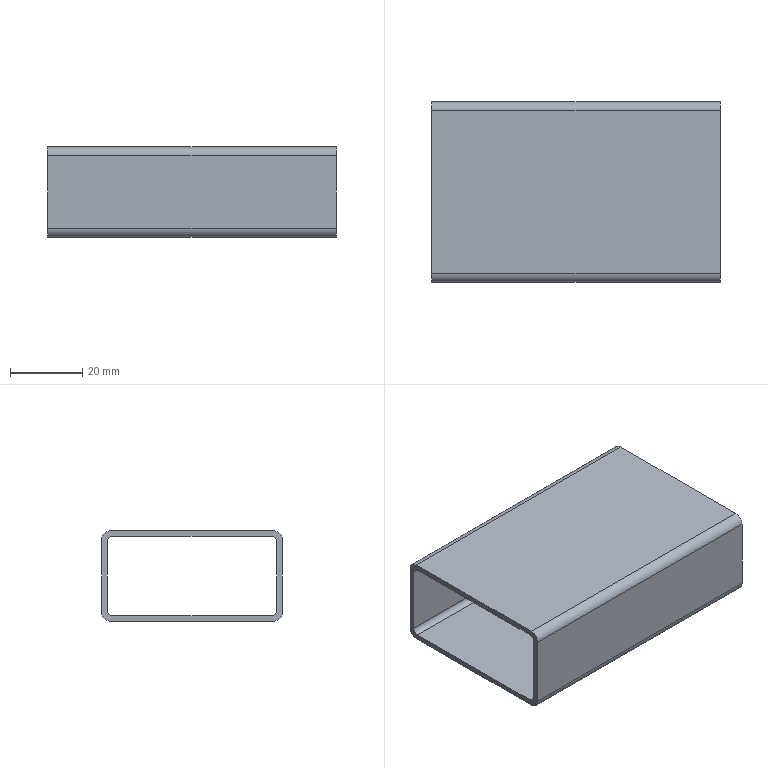Part | STEP file | 6100507 | 1 solid | 18 faces | box 80 x 50 x 25 mm | volume 17005 mm3 | plane 10 | cylinder 8 | commonest cylinder face diameters 3 x4 5 x4
STEP:
#1=CARTESIAN_POINT('',(0.,0.,0.));
#2=DIRECTION('',(0.,0.,1.));
#3=DIRECTION('',(1.,0.,0.));
#4=AXIS2_PLACEMENT_3D('',#1,#2,#3);
#5=CARTESIAN_POINT('',(-40.,22.,11.));
#6=VERTEX_POINT('',#5);
#7=CARTESIAN_POINT('',(-40.,-22.,11.));
#8=VERTEX_POINT('',#7);
#9=CARTESIAN_POINT('',(-40.,22.,11.));
#10=DIRECTION('',(0.,-1.,0.));
#11=VECTOR('',#10,1.);
#12=LINE('',#9,#11);
#13=CARTESIAN_POINT('',(-40.,25.,12.5));
#14=DIRECTION('',(1.,0.,0.));
#15=DIRECTION('',(0.,1.,0.));
#16=AXIS2_PLACEMENT_3D('',#13,#14,#15);
#17=PLANE('',#16);
#18=CARTESIAN_POINT('',(-3.,-1.5));
#19=DIRECTION('',(-1.,0.));
#20=VECTOR('',#19,1.);
#21=LINE('',#18,#20);
#22=(GEOMETRIC_REPRESENTATION_CONTEXT(2)PARAMETRIC_REPRESENTATION_CONTEXT()REPRESENTATION_CONTEXT('',''));
#23=DEFINITIONAL_REPRESENTATION('',(#21),#22);
#24=PCURVE('',#17,#23);
#25=CARTESIAN_POINT('',(-40.,22.,11.));
#26=DIRECTION('',(0.,0.,1.));
#27=DIRECTION('',(0.,-1.,0.));
#28=AXIS2_PLACEMENT_3D('',#25,#26,#27);
#29=PLANE('',#28);
#30=CARTESIAN_POINT('',(0.,0.));
#31=DIRECTION('',(1.,0.));
#32=VECTOR('',#31,1.);
#33=LINE('',#30,#32);
#34=(GEOMETRIC_REPRESENTATION_CONTEXT(2)PARAMETRIC_REPRESENTATION_CONTEXT()REPRESENTATION_CONTEXT('',''));
#35=DEFINITIONAL_REPRESENTATION('',(#33),#34);
#36=PCURVE('',#29,#35);
#37=SURFACE_CURVE('',#12,(#24,#36),.PCURVE_S1.);
#38=EDGE_CURVE('',#6,#8,#37,.T.);
#39=ORIENTED_EDGE('',*,*,#38,.T.);
#40=CARTESIAN_POINT('',(-40.,-23.5,9.5));
#41=VERTEX_POINT('',#40);
#42=CARTESIAN_POINT('',(-40.,-22.,9.5));
#43=DIRECTION('',(1.,0.,0.));
#44=DIRECTION('',(0.,1.,0.));
#45=AXIS2_PLACEMENT_3D('',#42,#43,#44);
#46=CIRCLE('',#45,1.5);
#47=CARTESIAN_POINT('',(-47.,-3.));
#48=DIRECTION('',(1.,0.));
#49=AXIS2_PLACEMENT_2D('',#47,#48);
#50=CIRCLE('',#49,1.5);
#51=(GEOMETRIC_REPRESENTATION_CONTEXT(2)PARAMETRIC_REPRESENTATION_CONTEXT()REPRESENTATION_CONTEXT('',''));
#52=DEFINITIONAL_REPRESENTATION('',(#50),#51);
#53=PCURVE('',#17,#52);
#54=CARTESIAN_POINT('',(-40.,-22.,9.5));
#55=DIRECTION('',(1.,0.,0.));
#56=DIRECTION('',(0.,1.,0.));
#57=AXIS2_PLACEMENT_3D('',#54,#55,#56);
#58=CYLINDRICAL_SURFACE('',#57,1.5);
#59=CARTESIAN_POINT('',(0.,0.));
#60=DIRECTION('',(1.,0.));
#61=VECTOR('',#60,1.);
#62=LINE('',#59,#61);
#63=(GEOMETRIC_REPRESENTATION_CONTEXT(2)PARAMETRIC_REPRESENTATION_CONTEXT()REPRESENTATION_CONTEXT('',''));
#64=DEFINITIONAL_REPRESENTATION('',(#62),#63);
#65=PCURVE('',#58,#64);
#66=SURFACE_CURVE('',#46,(#53,#65),.PCURVE_S1.);
#67=EDGE_CURVE('',#8,#41,#66,.T.);
#68=ORIENTED_EDGE('',*,*,#67,.T.);
#69=CARTESIAN_POINT('',(-40.,-23.5,-9.5));
#70=VERTEX_POINT('',#69);
#71=CARTESIAN_POINT('',(-40.,-23.5,9.5));
#72=DIRECTION('',(0.,0.,-1.));
#73=VECTOR('',#72,1.);
#74=LINE('',#71,#73);
#75=CARTESIAN_POINT('',(-48.5,-3.));
#76=DIRECTION('',(0.,-1.));
#77=VECTOR('',#76,1.);
#78=LINE('',#75,#77);
#79=(GEOMETRIC_REPRESENTATION_CONTEXT(2)PARAMETRIC_REPRESENTATION_CONTEXT()REPRESENTATION_CONTEXT('',''));
#80=DEFINITIONAL_REPRESENTATION('',(#78),#79);
#81=PCURVE('',#17,#80);
#82=CARTESIAN_POINT('',(-40.,-23.5,9.5));
#83=DIRECTION('',(0.,-1.,0.));
#84=DIRECTION('',(1.,0.,0.));
#85=AXIS2_PLACEMENT_3D('',#82,#83,#84);
#86=PLANE('',#85);
#87=CARTESIAN_POINT('',(0.,0.));
#88=DIRECTION('',(0.,-1.));
#89=VECTOR('',#88,1.);
#90=LINE('',#87,#89);
#91=(GEOMETRIC_REPRESENTATION_CONTEXT(2)PARAMETRIC_REPRESENTATION_CONTEXT()REPRESENTATION_CONTEXT('',''));
#92=DEFINITIONAL_REPRESENTATION('',(#90),#91);
#93=PCURVE('',#86,#92);
#94=SURFACE_CURVE('',#74,(#81,#93),.PCURVE_S1.);
#95=EDGE_CURVE('',#41,#70,#94,.T.);
#96=ORIENTED_EDGE('',*,*,#95,.T.);
#97=CARTESIAN_POINT('',(-40.,-22.,-11.));
#98=VERTEX_POINT('',#97);
#99=CARTESIAN_POINT('',(-40.,-22.,-9.5));
#100=DIRECTION('',(1.,0.,0.));
#101=DIRECTION('',(0.,1.,0.));
#102=AXIS2_PLACEMENT_3D('',#99,#100,#101);
#103=CIRCLE('',#102,1.5);
#104=CARTESIAN_POINT('',(-47.,-22.));
#105=DIRECTION('',(1.,0.));
#106=AXIS2_PLACEMENT_2D('',#104,#105);
#107=CIRCLE('',#106,1.5);
#108=(GEOMETRIC_REPRESENTATION_CONTEXT(2)PARAMETRIC_REPRESENTATION_CONTEXT()REPRESENTATION_CONTEXT('',''));
#109=DEFINITIONAL_REPRESENTATION('',(#107),#108);
#110=PCURVE('',#17,#109);
#111=CARTESIAN_POINT('',(-40.,-22.,-9.5));
#112=DIRECTION('',(1.,0.,0.));
#113=DIRECTION('',(0.,1.,0.));
#114=AXIS2_PLACEMENT_3D('',#111,#112,#113);
#115=CYLINDRICAL_SURFACE('',#114,1.5);
#116=CARTESIAN_POINT('',(0.,0.));
#117=DIRECTION('',(1.,0.));
#118=VECTOR('',#117,1.);
#119=LINE('',#116,#118);
#120=(GEOMETRIC_REPRESENTATION_CONTEXT(2)PARAMETRIC_REPRESENTATION_CONTEXT()REPRESENTATION_CONTEXT('',''));
#121=DEFINITIONAL_REPRESENTATION('',(#119),#120);
#122=PCURVE('',#115,#121);
#123=SURFACE_CURVE('',#103,(#110,#122),.PCURVE_S1.);
#124=EDGE_CURVE('',#70,#98,#123,.T.);
#125=ORIENTED_EDGE('',*,*,#124,.T.);
#126=CARTESIAN_POINT('',(-40.,22.,-11.));
#127=VERTEX_POINT('',#126);
#128=CARTESIAN_POINT('',(-40.,22.,-11.));
#129=DIRECTION('',(0.,1.,0.));
#130=VECTOR('',#129,1.);
#131=LINE('',#128,#130);
#132=CARTESIAN_POINT('',(-3.,-23.5));
#133=DIRECTION('',(1.,0.));
#134=VECTOR('',#133,1.);
#135=LINE('',#132,#134);
#136=(GEOMETRIC_REPRESENTATION_CONTEXT(2)PARAMETRIC_REPRESENTATION_CONTEXT()REPRESENTATION_CONTEXT('',''));
#137=DEFINITIONAL_REPRESENTATION('',(#135),#136);
#138=PCURVE('',#17,#137);
#139=CARTESIAN_POINT('',(-40.,22.,-11.));
#140=DIRECTION('',(0.,0.,-1.));
#141=DIRECTION('',(0.,1.,0.));
#142=AXIS2_PLACEMENT_3D('',#139,#140,#141);
#143=PLANE('',#142);
#144=CARTESIAN_POINT('',(0.,0.));
#145=DIRECTION('',(1.,0.));
#146=VECTOR('',#145,1.);
#147=LINE('',#144,#146);
#148=(GEOMETRIC_REPRESENTATION_CONTEXT(2)PARAMETRIC_REPRESENTATION_CONTEXT()REPRESENTATION_CONTEXT('',''));
#149=DEFINITIONAL_REPRESENTATION('',(#147),#148);
#150=PCURVE('',#143,#149);
#151=SURFACE_CURVE('',#131,(#138,#150),.PCURVE_S1.);
#152=EDGE_CURVE('',#98,#127,#151,.T.);
#153=ORIENTED_EDGE('',*,*,#152,.T.);
#154=CARTESIAN_POINT('',(-40.,23.5,-9.5));
#155=VERTEX_POINT('',#154);
#156=CARTESIAN_POINT('',(-40.,22.,-9.5));
#157=DIRECTION('',(1.,0.,0.));
#158=DIRECTION('',(0.,-1.,0.));
#159=AXIS2_PLACEMENT_3D('',#156,#157,#158);
#160=CIRCLE('',#159,1.5);
#161=CARTESIAN_POINT('',(-3.,-22.));
#162=DIRECTION('',(-1.,0.));
#163=AXIS2_PLACEMENT_2D('',#161,#162);
#164=CIRCLE('',#163,1.5);
#165=(GEOMETRIC_REPRESENTATION_CONTEXT(2)PARAMETRIC_REPRESENTATION_CONTEXT()REPRESENTATION_CONTEXT('',''));
#166=DEFINITIONAL_REPRESENTATION('',(#164),#165);
#167=PCURVE('',#17,#166);
#168=CARTESIAN_POINT('',(-40.,22.,-9.5));
#169=DIRECTION('',(1.,0.,0.));
#170=DIRECTION('',(0.,1.,0.));
#171=AXIS2_PLACEMENT_3D('',#168,#169,#170);
#172=CYLINDRICAL_SURFACE('',#171,1.5);
#173=CARTESIAN_POINT('',(3.142,0.));
#174=DIRECTION('',(1.,0.));
#175=VECTOR('',#174,1.);
#176=LINE('',#173,#175);
#177=(GEOMETRIC_REPRESENTATION_CONTEXT(2)PARAMETRIC_REPRESENTATION_CONTEXT()REPRESENTATION_CONTEXT('',''));
#178=DEFINITIONAL_REPRESENTATION('',(#176),#177);
#179=PCURVE('',#172,#178);
#180=SURFACE_CURVE('',#160,(#167,#179),.PCURVE_S1.);
#181=EDGE_CURVE('',#127,#155,#180,.T.);
#182=ORIENTED_EDGE('',*,*,#181,.T.);
#183=CARTESIAN_POINT('',(-40.,23.5,9.5));
#184=VERTEX_POINT('',#183);
#185=CARTESIAN_POINT('',(-40.,23.5,9.5));
#186=DIRECTION('',(0.,0.,1.));
#187=VECTOR('',#186,1.);
#188=LINE('',#185,#187);
#189=CARTESIAN_POINT('',(-1.5,-3.));
#190=DIRECTION('',(0.,1.));
#191=VECTOR('',#190,1.);
#192=LINE('',#189,#191);
#193=(GEOMETRIC_REPRESENTATION_CONTEXT(2)PARAMETRIC_REPRESENTATION_CONTEXT()REPRESENTATION_CONTEXT('',''));
#194=DEFINITIONAL_REPRESENTATION('',(#192),#193);
#195=PCURVE('',#17,#194);
#196=CARTESIAN_POINT('',(-40.,23.5,9.5));
#197=DIRECTION('',(0.,1.,0.));
#198=DIRECTION('',(-1.,0.,0.));
#199=AXIS2_PLACEMENT_3D('',#196,#197,#198);
#200=PLANE('',#199);
#201=CARTESIAN_POINT('',(0.,0.));
#202=DIRECTION('',(0.,1.));
#203=VECTOR('',#202,1.);
#204=LINE('',#201,#203);
#205=(GEOMETRIC_REPRESENTATION_CONTEXT(2)PARAMETRIC_REPRESENTATION_CONTEXT()REPRESENTATION_CONTEXT('',''));
#206=DEFINITIONAL_REPRESENTATION('',(#204),#205);
#207=PCURVE('',#200,#206);
#208=SURFACE_CURVE('',#188,(#195,#207),.PCURVE_S1.);
#209=EDGE_CURVE('',#155,#184,#208,.T.);
#210=ORIENTED_EDGE('',*,*,#209,.T.);
#211=CARTESIAN_POINT('',(-40.,22.,9.5));
#212=DIRECTION('',(1.,0.,0.));
#213=DIRECTION('',(0.,1.,0.));
#214=AXIS2_PLACEMENT_3D('',#211,#212,#213);
#215=CIRCLE('',#214,1.5);
#216=CARTESIAN_POINT('',(-3.,-3.));
#217=DIRECTION('',(1.,0.));
#218=AXIS2_PLACEMENT_2D('',#216,#217);
#219=CIRCLE('',#218,1.5);
#220=(GEOMETRIC_REPRESENTATION_CONTEXT(2)PARAMETRIC_REPRESENTATION_CONTEXT()REPRESENTATION_CONTEXT('',''));
#221=DEFINITIONAL_REPRESENTATION('',(#219),#220);
#222=PCURVE('',#17,#221);
#223=CARTESIAN_POINT('',(-40.,22.,9.5));
#224=DIRECTION('',(1.,0.,0.));
#225=DIRECTION('',(0.,1.,0.));
#226=AXIS2_PLACEMENT_3D('',#223,#224,#225);
#227=CYLINDRICAL_SURFACE('',#226,1.5);
#228=CARTESIAN_POINT('',(0.,0.));
#229=DIRECTION('',(1.,0.));
#230=VECTOR('',#229,1.);
#231=LINE('',#228,#230);
#232=(GEOMETRIC_REPRESENTATION_CONTEXT(2)PARAMETRIC_REPRESENTATION_CONTEXT()REPRESENTATION_CONTEXT('',''));
#233=DEFINITIONAL_REPRESENTATION('',(#231),#232);
#234=PCURVE('',#227,#233);
#235=SURFACE_CURVE('',#215,(#222,#234),.PCURVE_S1.);
#236=EDGE_CURVE('',#184,#6,#235,.T.);
#237=ORIENTED_EDGE('',*,*,#236,.T.);
#238=EDGE_LOOP('',(#39,#68,#96,#125,#153,#182,#210,#237));
#239=FACE_BOUND('',#238,.T.);
#240=CARTESIAN_POINT('',(-40.,-25.,10.));
#241=VERTEX_POINT('',#240);
#242=CARTESIAN_POINT('',(-40.,-25.,-10.));
#243=VERTEX_POINT('',#242);
#244=CARTESIAN_POINT('',(-40.,-25.,12.5));
#245=DIRECTION('',(0.,0.,-1.));
#246=VECTOR('',#245,1.);
#247=LINE('',#244,#246);
#248=CARTESIAN_POINT('',(-50.,0.));
#249=DIRECTION('',(0.,-1.));
#250=VECTOR('',#249,1.);
#251=LINE('',#248,#250);
#252=(GEOMETRIC_REPRESENTATION_CONTEXT(2)PARAMETRIC_REPRESENTATION_CONTEXT()REPRESENTATION_CONTEXT('',''));
#253=DEFINITIONAL_REPRESENTATION('',(#251),#252);
#254=PCURVE('',#17,#253);
#255=CARTESIAN_POINT('',(-40.,-25.,12.5));
#256=DIRECTION('',(0.,1.,0.));
#257=DIRECTION('',(-1.,0.,0.));
#258=AXIS2_PLACEMENT_3D('',#255,#256,#257);
#259=PLANE('',#258);
#260=CARTESIAN_POINT('',(0.,0.));
#261=DIRECTION('',(0.,-1.));
#262=VECTOR('',#261,1.);
#263=LINE('',#260,#262);
#264=(GEOMETRIC_REPRESENTATION_CONTEXT(2)PARAMETRIC_REPRESENTATION_CONTEXT()REPRESENTATION_CONTEXT('',''));
#265=DEFINITIONAL_REPRESENTATION('',(#263),#264);
#266=PCURVE('',#259,#265);
#267=SURFACE_CURVE('',#247,(#254,#266),.PCURVE_S1.);
#268=EDGE_CURVE('',#241,#243,#267,.T.);
#269=ORIENTED_EDGE('',*,*,#268,.F.);
#270=CARTESIAN_POINT('',(-40.,-22.5,12.5));
#271=VERTEX_POINT('',#270);
#272=CARTESIAN_POINT('',(-40.,-22.5,10.));
#273=DIRECTION('',(-1.,0.,0.));
#274=DIRECTION('',(0.,1.,0.));
#275=AXIS2_PLACEMENT_3D('',#272,#273,#274);
#276=CIRCLE('',#275,2.5);
#277=CARTESIAN_POINT('',(-45.,-2.5));
#278=CARTESIAN_POINT('',(-45.,-6.83));
#279=CARTESIAN_POINT('',(-48.75,-4.665));
#280=CARTESIAN_POINT('',(-52.5,-2.5));
#281=CARTESIAN_POINT('',(-48.75,-0.3349));
#282=CARTESIAN_POINT('',(-45.,1.83));
#283=CARTESIAN_POINT('',(-45.,-2.5));
#284=(BOUNDED_CURVE()B_SPLINE_CURVE(2,(#277,#278,#279,#280,#281,#282,#283),.UNSPECIFIED.,.T.,.F.)B_SPLINE_CURVE_WITH_KNOTS((1,2,2,2,2,1),(-2.094,0.,2.094,4.189,6.283,8.378),.UNSPECIFIED.)CURVE()GEOMETRIC_REPRESENTATION_ITEM()RATIONAL_B_SPLINE_CURVE((1.,0.5,1.,0.5,1.,0.5,1.))REPRESENTATION_ITEM(''));
#285=(GEOMETRIC_REPRESENTATION_CONTEXT(2)PARAMETRIC_REPRESENTATION_CONTEXT()REPRESENTATION_CONTEXT('',''));
#286=DEFINITIONAL_REPRESENTATION('',(#284),#285);
#287=PCURVE('',#17,#286);
#288=CARTESIAN_POINT('',(-40.,-22.5,10.));
#289=DIRECTION('',(-1.,0.,0.));
#290=DIRECTION('',(0.,-1.,0.));
#291=AXIS2_PLACEMENT_3D('',#288,#289,#290);
#292=CYLINDRICAL_SURFACE('',#291,2.5);
#293=CARTESIAN_POINT('',(-3.142,0.));
#294=DIRECTION('',(1.,0.));
#295=VECTOR('',#294,1.);
#296=LINE('',#293,#295);
#297=(GEOMETRIC_REPRESENTATION_CONTEXT(2)PARAMETRIC_REPRESENTATION_CONTEXT()REPRESENTATION_CONTEXT('',''));
#298=DEFINITIONAL_REPRESENTATION('',(#296),#297);
#299=PCURVE('',#292,#298);
#300=SURFACE_CURVE('',#276,(#287,#299),.PCURVE_S1.);
#301=EDGE_CURVE('',#241,#271,#300,.T.);
#302=ORIENTED_EDGE('',*,*,#301,.T.);
#303=CARTESIAN_POINT('',(-40.,22.5,12.5));
#304=VERTEX_POINT('',#303);
#305=CARTESIAN_POINT('',(-40.,25.,12.5));
#306=DIRECTION('',(0.,-1.,0.));
#307=VECTOR('',#306,1.);
#308=LINE('',#305,#307);
#309=CARTESIAN_POINT('',(0.,0.));
#310=DIRECTION('',(-1.,0.));
#311=VECTOR('',#310,1.);
#312=LINE('',#309,#311);
#313=(GEOMETRIC_REPRESENTATION_CONTEXT(2)PARAMETRIC_REPRESENTATION_CONTEXT()REPRESENTATION_CONTEXT('',''));
#314=DEFINITIONAL_REPRESENTATION('',(#312),#313);
#315=PCURVE('',#17,#314);
#316=CARTESIAN_POINT('',(-40.,-25.,12.5));
#317=DIRECTION('',(0.,0.,1.));
#318=DIRECTION('',(1.,0.,0.));
#319=AXIS2_PLACEMENT_3D('',#316,#317,#318);
#320=PLANE('',#319);
#321=CARTESIAN_POINT('',(0.,50.));
#322=DIRECTION('',(0.,-1.));
#323=VECTOR('',#322,1.);
#324=LINE('',#321,#323);
#325=(GEOMETRIC_REPRESENTATION_CONTEXT(2)PARAMETRIC_REPRESENTATION_CONTEXT()REPRESENTATION_CONTEXT('',''));
#326=DEFINITIONAL_REPRESENTATION('',(#324),#325);
#327=PCURVE('',#320,#326);
#328=SURFACE_CURVE('',#308,(#315,#327),.PCURVE_S1.);
#329=EDGE_CURVE('',#304,#271,#328,.T.);
#330=ORIENTED_EDGE('',*,*,#329,.F.);
#331=CARTESIAN_POINT('',(-40.,25.,10.));
#332=VERTEX_POINT('',#331);
#333=CARTESIAN_POINT('',(-40.,22.5,10.));
#334=DIRECTION('',(-1.,0.,0.));
#335=DIRECTION('',(0.,1.,0.));
#336=AXIS2_PLACEMENT_3D('',#333,#334,#335);
#337=CIRCLE('',#336,2.5);
#338=CARTESIAN_POINT('',(0.,-2.5));
#339=CARTESIAN_POINT('',(0.,-6.83));
#340=CARTESIAN_POINT('',(-3.75,-4.665));
#341=CARTESIAN_POINT('',(-7.5,-2.5));
#342=CARTESIAN_POINT('',(-3.75,-0.3349));
#343=CARTESIAN_POINT('',(0.,1.83));
#344=CARTESIAN_POINT('',(0.,-2.5));
#345=(BOUNDED_CURVE()B_SPLINE_CURVE(2,(#338,#339,#340,#341,#342,#343,#344),.UNSPECIFIED.,.T.,.F.)B_SPLINE_CURVE_WITH_KNOTS((1,2,2,2,2,1),(-2.094,0.,2.094,4.189,6.283,8.378),.UNSPECIFIED.)CURVE()GEOMETRIC_REPRESENTATION_ITEM()RATIONAL_B_SPLINE_CURVE((1.,0.5,1.,0.5,1.,0.5,1.))REPRESENTATION_ITEM(''));
#346=(GEOMETRIC_REPRESENTATION_CONTEXT(2)PARAMETRIC_REPRESENTATION_CONTEXT()REPRESENTATION_CONTEXT('',''));
#347=DEFINITIONAL_REPRESENTATION('',(#345),#346);
#348=PCURVE('',#17,#347);
#349=CARTESIAN_POINT('',(-40.,22.5,10.));
#350=DIRECTION('',(1.,0.,0.));
#351=DIRECTION('',(0.,0.,-1.));
#352=AXIS2_PLACEMENT_3D('',#349,#350,#351);
#353=CYLINDRICAL_SURFACE('',#352,2.5);
#354=CARTESIAN_POINT('',(7.854,0.));
#355=DIRECTION('',(-1.,0.));
#356=VECTOR('',#355,1.);
#357=LINE('',#354,#356);
#358=(GEOMETRIC_REPRESENTATION_CONTEXT(2)PARAMETRIC_REPRESENTATION_CONTEXT()REPRESENTATION_CONTEXT('',''));
#359=DEFINITIONAL_REPRESENTATION('',(#357),#358);
#360=PCURVE('',#353,#359);
#361=SURFACE_CURVE('',#337,(#348,#360),.PCURVE_S1.);
#362=EDGE_CURVE('',#304,#332,#361,.T.);
#363=ORIENTED_EDGE('',*,*,#362,.T.);
#364=CARTESIAN_POINT('',(-40.,25.,-10.));
#365=VERTEX_POINT('',#364);
#366=CARTESIAN_POINT('',(-40.,25.,12.5));
#367=DIRECTION('',(0.,0.,-1.));
#368=VECTOR('',#367,1.);
#369=LINE('',#366,#368);
#370=CARTESIAN_POINT('',(0.,0.));
#371=DIRECTION('',(0.,-1.));
#372=VECTOR('',#371,1.);
#373=LINE('',#370,#372);
#374=(GEOMETRIC_REPRESENTATION_CONTEXT(2)PARAMETRIC_REPRESENTATION_CONTEXT()REPRESENTATION_CONTEXT('',''));
#375=DEFINITIONAL_REPRESENTATION('',(#373),#374);
#376=PCURVE('',#17,#375);
#377=CARTESIAN_POINT('',(-40.,25.,12.5));
#378=DIRECTION('',(0.,-1.,0.));
#379=DIRECTION('',(0.,0.,-1.));
#380=AXIS2_PLACEMENT_3D('',#377,#378,#379);
#381=PLANE('',#380);
#382=CARTESIAN_POINT('',(0.,0.));
#383=DIRECTION('',(1.,0.));
#384=VECTOR('',#383,1.);
#385=LINE('',#382,#384);
#386=(GEOMETRIC_REPRESENTATION_CONTEXT(2)PARAMETRIC_REPRESENTATION_CONTEXT()REPRESENTATION_CONTEXT('',''));
#387=DEFINITIONAL_REPRESENTATION('',(#385),#386);
#388=PCURVE('',#381,#387);
#389=SURFACE_CURVE('',#369,(#376,#388),.PCURVE_S1.);
#390=EDGE_CURVE('',#332,#365,#389,.T.);
#391=ORIENTED_EDGE('',*,*,#390,.T.);
#392=CARTESIAN_POINT('',(-40.,22.5,-12.5));
#393=VERTEX_POINT('',#392);
#394=CARTESIAN_POINT('',(-40.,22.5,-10.));
#395=DIRECTION('',(-1.,0.,0.));
#396=DIRECTION('',(0.,1.,0.));
#397=AXIS2_PLACEMENT_3D('',#394,#395,#396);
#398=CIRCLE('',#397,2.5);
#399=CARTESIAN_POINT('',(0.,-22.5));
#400=CARTESIAN_POINT('',(0.,-26.83));
#401=CARTESIAN_POINT('',(-3.75,-24.665));
#402=CARTESIAN_POINT('',(-7.5,-22.5));
#403=CARTESIAN_POINT('',(-3.75,-20.335));
#404=CARTESIAN_POINT('',(0.,-18.17));
#405=CARTESIAN_POINT('',(0.,-22.5));
#406=(BOUNDED_CURVE()B_SPLINE_CURVE(2,(#399,#400,#401,#402,#403,#404,#405),.UNSPECIFIED.,.T.,.F.)B_SPLINE_CURVE_WITH_KNOTS((1,2,2,2,2,1),(-2.094,0.,2.094,4.189,6.283,8.378),.UNSPECIFIED.)CURVE()GEOMETRIC_REPRESENTATION_ITEM()RATIONAL_B_SPLINE_CURVE((1.,0.5,1.,0.5,1.,0.5,1.))REPRESENTATION_ITEM(''));
#407=(GEOMETRIC_REPRESENTATION_CONTEXT(2)PARAMETRIC_REPRESENTATION_CONTEXT()REPRESENTATION_CONTEXT('',''));
#408=DEFINITIONAL_REPRESENTATION('',(#406),#407);
#409=PCURVE('',#17,#408);
#410=CARTESIAN_POINT('',(-40.,22.5,-10.));
#411=DIRECTION('',(-1.,0.,0.));
#412=DIRECTION('',(0.,0.,1.));
#413=AXIS2_PLACEMENT_3D('',#410,#411,#412);
#414=CYLINDRICAL_SURFACE('',#413,2.5);
#415=CARTESIAN_POINT('',(1.571,0.));
#416=DIRECTION('',(1.,0.));
#417=VECTOR('',#416,1.);
#418=LINE('',#415,#417);
#419=(GEOMETRIC_REPRESENTATION_CONTEXT(2)PARAMETRIC_REPRESENTATION_CONTEXT()REPRESENTATION_CONTEXT('',''));
#420=DEFINITIONAL_REPRESENTATION('',(#418),#419);
#421=PCURVE('',#414,#420);
#422=SURFACE_CURVE('',#398,(#409,#421),.PCURVE_S1.);
#423=EDGE_CURVE('',#365,#393,#422,.T.);
#424=ORIENTED_EDGE('',*,*,#423,.T.);
#425=CARTESIAN_POINT('',(-40.,-22.5,-12.5));
#426=VERTEX_POINT('',#425);
#427=CARTESIAN_POINT('',(-40.,25.,-12.5));
#428=DIRECTION('',(0.,-1.,0.));
#429=VECTOR('',#428,1.);
#430=LINE('',#427,#429);
#431=CARTESIAN_POINT('',(0.,-25.));
#432=DIRECTION('',(-1.,0.));
#433=VECTOR('',#432,1.);
#434=LINE('',#431,#433);
#435=(GEOMETRIC_REPRESENTATION_CONTEXT(2)PARAMETRIC_REPRESENTATION_CONTEXT()REPRESENTATION_CONTEXT('',''));
#436=DEFINITIONAL_REPRESENTATION('',(#434),#435);
#437=PCURVE('',#17,#436);
#438=CARTESIAN_POINT('',(-40.,-25.,-12.5));
#439=DIRECTION('',(0.,0.,1.));
#440=DIRECTION('',(1.,0.,0.));
#441=AXIS2_PLACEMENT_3D('',#438,#439,#440);
#442=PLANE('',#441);
#443=CARTESIAN_POINT('',(0.,50.));
#444=DIRECTION('',(0.,-1.));
#445=VECTOR('',#444,1.);
#446=LINE('',#443,#445);
#447=(GEOMETRIC_REPRESENTATION_CONTEXT(2)PARAMETRIC_REPRESENTATION_CONTEXT()REPRESENTATION_CONTEXT('',''));
#448=DEFINITIONAL_REPRESENTATION('',(#446),#447);
#449=PCURVE('',#442,#448);
#450=SURFACE_CURVE('',#430,(#437,#449),.PCURVE_S1.);
#451=EDGE_CURVE('',#393,#426,#450,.T.);
#452=ORIENTED_EDGE('',*,*,#451,.T.);
#453=CARTESIAN_POINT('',(-40.,-22.5,-10.));
#454=DIRECTION('',(-1.,0.,0.));
#455=DIRECTION('',(0.,1.,0.));
#456=AXIS2_PLACEMENT_3D('',#453,#454,#455);
#457=CIRCLE('',#456,2.5);
#458=CARTESIAN_POINT('',(-45.,-22.5));
#459=CARTESIAN_POINT('',(-45.,-26.83));
#460=CARTESIAN_POINT('',(-48.75,-24.665));
#461=CARTESIAN_POINT('',(-52.5,-22.5));
#462=CARTESIAN_POINT('',(-48.75,-20.335));
#463=CARTESIAN_POINT('',(-45.,-18.17));
#464=CARTESIAN_POINT('',(-45.,-22.5));
#465=(BOUNDED_CURVE()B_SPLINE_CURVE(2,(#458,#459,#460,#461,#462,#463,#464),.UNSPECIFIED.,.T.,.F.)B_SPLINE_CURVE_WITH_KNOTS((1,2,2,2,2,1),(-2.094,0.,2.094,4.189,6.283,8.378),.UNSPECIFIED.)CURVE()GEOMETRIC_REPRESENTATION_ITEM()RATIONAL_B_SPLINE_CURVE((1.,0.5,1.,0.5,1.,0.5,1.))REPRESENTATION_ITEM(''));
#466=(GEOMETRIC_REPRESENTATION_CONTEXT(2)PARAMETRIC_REPRESENTATION_CONTEXT()REPRESENTATION_CONTEXT('',''));
#467=DEFINITIONAL_REPRESENTATION('',(#465),#466);
#468=PCURVE('',#17,#467);
#469=CARTESIAN_POINT('',(-40.,-22.5,-10.));
#470=DIRECTION('',(1.,0.,0.));
#471=DIRECTION('',(0.,1.,0.));
#472=AXIS2_PLACEMENT_3D('',#469,#470,#471);
#473=CYLINDRICAL_SURFACE('',#472,2.5);
#474=CARTESIAN_POINT('',(6.283,0.));
#475=DIRECTION('',(-1.,0.));
#476=VECTOR('',#475,1.);
#477=LINE('',#474,#476);
#478=(GEOMETRIC_REPRESENTATION_CONTEXT(2)PARAMETRIC_REPRESENTATION_CONTEXT()REPRESENTATION_CONTEXT('',''));
#479=DEFINITIONAL_REPRESENTATION('',(#477),#478);
#480=PCURVE('',#473,#479);
#481=SURFACE_CURVE('',#457,(#468,#480),.PCURVE_S1.);
#482=EDGE_CURVE('',#426,#243,#481,.T.);
#483=ORIENTED_EDGE('',*,*,#482,.T.);
#484=EDGE_LOOP('',(#269,#302,#330,#363,#391,#424,#452,#483));
#485=FACE_BOUND('',#484,.T.);
#486=ADVANCED_FACE('',(#239,#485),#17,.F.);
#487=CARTESIAN_POINT('',(40.,-25.,10.));
#488=VERTEX_POINT('',#487);
#489=CARTESIAN_POINT('',(40.,-25.,-10.));
#490=VERTEX_POINT('',#489);
#491=CARTESIAN_POINT('',(40.,-25.,12.5));
#492=DIRECTION('',(0.,0.,-1.));
#493=VECTOR('',#492,1.);
#494=LINE('',#491,#493);
#495=CARTESIAN_POINT('',(-80.,0.));
#496=DIRECTION('',(0.,-1.));
#497=VECTOR('',#496,1.);
#498=LINE('',#495,#497);
#499=(GEOMETRIC_REPRESENTATION_CONTEXT(2)PARAMETRIC_REPRESENTATION_CONTEXT()REPRESENTATION_CONTEXT('',''));
#500=DEFINITIONAL_REPRESENTATION('',(#498),#499);
#501=PCURVE('',#259,#500);
#502=CARTESIAN_POINT('',(40.,25.,12.5));
#503=DIRECTION('',(-1.,0.,0.));
#504=DIRECTION('',(0.,-1.,0.));
#505=AXIS2_PLACEMENT_3D('',#502,#503,#504);
#506=PLANE('',#505);
#507=CARTESIAN_POINT('',(50.,0.));
#508=DIRECTION('',(0.,-1.));
#509=VECTOR('',#508,1.);
#510=LINE('',#507,#509);
#511=(GEOMETRIC_REPRESENTATION_CONTEXT(2)PARAMETRIC_REPRESENTATION_CONTEXT()REPRESENTATION_CONTEXT('',''));
#512=DEFINITIONAL_REPRESENTATION('',(#510),#511);
#513=PCURVE('',#506,#512);
#514=SURFACE_CURVE('',#494,(#501,#513),.PCURVE_S1.);
#515=EDGE_CURVE('',#488,#490,#514,.T.);
#516=ORIENTED_EDGE('',*,*,#515,.F.);
#517=CARTESIAN_POINT('',(-40.,-25.,10.));
#518=DIRECTION('',(-1.,0.,0.));
#519=VECTOR('',#518,1.);
#520=LINE('',#517,#519);
#521=CARTESIAN_POINT('',(0.,-2.5));
#522=DIRECTION('',(1.,0.));
#523=VECTOR('',#522,1.);
#524=LINE('',#521,#523);
#525=(GEOMETRIC_REPRESENTATION_CONTEXT(2)PARAMETRIC_REPRESENTATION_CONTEXT()REPRESENTATION_CONTEXT('',''));
#526=DEFINITIONAL_REPRESENTATION('',(#524),#525);
#527=PCURVE('',#259,#526);
#528=CARTESIAN_POINT('',(0.,0.));
#529=DIRECTION('',(0.,1.));
#530=VECTOR('',#529,1.);
#531=LINE('',#528,#530);
#532=(GEOMETRIC_REPRESENTATION_CONTEXT(2)PARAMETRIC_REPRESENTATION_CONTEXT()REPRESENTATION_CONTEXT('',''));
#533=DEFINITIONAL_REPRESENTATION('',(#531),#532);
#534=PCURVE('',#292,#533);
#535=SURFACE_CURVE('',#520,(#527,#534),.PCURVE_S1.);
#536=EDGE_CURVE('',#488,#241,#535,.T.);
#537=ORIENTED_EDGE('',*,*,#536,.T.);
#538=ORIENTED_EDGE('',*,*,#268,.T.);
#539=CARTESIAN_POINT('',(-40.,-25.,-10.));
#540=DIRECTION('',(1.,0.,0.));
#541=VECTOR('',#540,1.);
#542=LINE('',#539,#541);
#543=CARTESIAN_POINT('',(0.,-22.5));
#544=DIRECTION('',(-1.,0.));
#545=VECTOR('',#544,1.);
#546=LINE('',#543,#545);
#547=(GEOMETRIC_REPRESENTATION_CONTEXT(2)PARAMETRIC_REPRESENTATION_CONTEXT()REPRESENTATION_CONTEXT('',''));
#548=DEFINITIONAL_REPRESENTATION('',(#546),#547);
#549=PCURVE('',#259,#548);
#550=CARTESIAN_POINT('',(3.142,0.));
#551=DIRECTION('',(0.,1.));
#552=VECTOR('',#551,1.);
#553=LINE('',#550,#552);
#554=(GEOMETRIC_REPRESENTATION_CONTEXT(2)PARAMETRIC_REPRESENTATION_CONTEXT()REPRESENTATION_CONTEXT('',''));
#555=DEFINITIONAL_REPRESENTATION('',(#553),#554);
#556=PCURVE('',#473,#555);
#557=SURFACE_CURVE('',#542,(#549,#556),.PCURVE_S1.);
#558=EDGE_CURVE('',#243,#490,#557,.T.);
#559=ORIENTED_EDGE('',*,*,#558,.T.);
#560=EDGE_LOOP('',(#516,#537,#538,#559));
#561=FACE_BOUND('',#560,.T.);
#562=ADVANCED_FACE('',(#561),#259,.F.);
#563=CARTESIAN_POINT('',(40.,-23.5,9.5));
#564=VERTEX_POINT('',#563);
#565=CARTESIAN_POINT('',(40.,-23.5,-9.5));
#566=VERTEX_POINT('',#565);
#567=CARTESIAN_POINT('',(40.,-23.5,9.5));
#568=DIRECTION('',(0.,0.,-1.));
#569=VECTOR('',#568,1.);
#570=LINE('',#567,#569);
#571=CARTESIAN_POINT('',(48.5,-3.));
#572=DIRECTION('',(0.,-1.));
#573=VECTOR('',#572,1.);
#574=LINE('',#571,#573);
#575=(GEOMETRIC_REPRESENTATION_CONTEXT(2)PARAMETRIC_REPRESENTATION_CONTEXT()REPRESENTATION_CONTEXT('',''));
#576=DEFINITIONAL_REPRESENTATION('',(#574),#575);
#577=PCURVE('',#506,#576);
#578=CARTESIAN_POINT('',(80.,0.));
#579=DIRECTION('',(0.,-1.));
#580=VECTOR('',#579,1.);
#581=LINE('',#578,#580);
#582=(GEOMETRIC_REPRESENTATION_CONTEXT(2)PARAMETRIC_REPRESENTATION_CONTEXT()REPRESENTATION_CONTEXT('',''));
#583=DEFINITIONAL_REPRESENTATION('',(#581),#582);
#584=PCURVE('',#86,#583);
#585=SURFACE_CURVE('',#570,(#577,#584),.PCURVE_S1.);
#586=EDGE_CURVE('',#564,#566,#585,.T.);
#587=ORIENTED_EDGE('',*,*,#586,.F.);
#588=CARTESIAN_POINT('',(40.,-22.,11.));
#589=VERTEX_POINT('',#588);
#590=CARTESIAN_POINT('',(40.,-22.,9.5));
#591=DIRECTION('',(1.,0.,0.));
#592=DIRECTION('',(0.,1.,0.));
#593=AXIS2_PLACEMENT_3D('',#590,#591,#592);
#594=CIRCLE('',#593,1.5);
#595=CARTESIAN_POINT('',(45.5,-3.));
#596=CARTESIAN_POINT('',(45.5,-0.4019));
#597=CARTESIAN_POINT('',(47.75,-1.701));
#598=CARTESIAN_POINT('',(50.,-3.));
#599=CARTESIAN_POINT('',(47.75,-4.299));
#600=CARTESIAN_POINT('',(45.5,-5.598));
#601=CARTESIAN_POINT('',(45.5,-3.));
#602=(BOUNDED_CURVE()B_SPLINE_CURVE(2,(#595,#596,#597,#598,#599,#600,#601),.UNSPECIFIED.,.T.,.F.)B_SPLINE_CURVE_WITH_KNOTS((1,2,2,2,2,1),(-2.094,0.,2.094,4.189,6.283,8.378),.UNSPECIFIED.)CURVE()GEOMETRIC_REPRESENTATION_ITEM()RATIONAL_B_SPLINE_CURVE((1.,0.5,1.,0.5,1.,0.5,1.))REPRESENTATION_ITEM(''));
#603=(GEOMETRIC_REPRESENTATION_CONTEXT(2)PARAMETRIC_REPRESENTATION_CONTEXT()REPRESENTATION_CONTEXT('',''));
#604=DEFINITIONAL_REPRESENTATION('',(#602),#603);
#605=PCURVE('',#506,#604);
#606=CARTESIAN_POINT('',(0.,80.));
#607=DIRECTION('',(1.,0.));
#608=VECTOR('',#607,1.);
#609=LINE('',#606,#608);
#610=(GEOMETRIC_REPRESENTATION_CONTEXT(2)PARAMETRIC_REPRESENTATION_CONTEXT()REPRESENTATION_CONTEXT('',''));
#611=DEFINITIONAL_REPRESENTATION('',(#609),#610);
#612=PCURVE('',#58,#611);
#613=SURFACE_CURVE('',#594,(#605,#612),.PCURVE_S1.);
#614=EDGE_CURVE('',#589,#564,#613,.T.);
#615=ORIENTED_EDGE('',*,*,#614,.F.);
#616=CARTESIAN_POINT('',(40.,22.,11.));
#617=VERTEX_POINT('',#616);
#618=CARTESIAN_POINT('',(40.,22.,11.));
#619=DIRECTION('',(0.,-1.,0.));
#620=VECTOR('',#619,1.);
#621=LINE('',#618,#620);
#622=CARTESIAN_POINT('',(3.,-1.5));
#623=DIRECTION('',(1.,0.));
#624=VECTOR('',#623,1.);
#625=LINE('',#622,#624);
#626=(GEOMETRIC_REPRESENTATION_CONTEXT(2)PARAMETRIC_REPRESENTATION_CONTEXT()REPRESENTATION_CONTEXT('',''));
#627=DEFINITIONAL_REPRESENTATION('',(#625),#626);
#628=PCURVE('',#506,#627);
#629=CARTESIAN_POINT('',(0.,80.));
#630=DIRECTION('',(1.,0.));
#631=VECTOR('',#630,1.);
#632=LINE('',#629,#631);
#633=(GEOMETRIC_REPRESENTATION_CONTEXT(2)PARAMETRIC_REPRESENTATION_CONTEXT()REPRESENTATION_CONTEXT('',''));
#634=DEFINITIONAL_REPRESENTATION('',(#632),#633);
#635=PCURVE('',#29,#634);
#636=SURFACE_CURVE('',#621,(#628,#635),.PCURVE_S1.);
#637=EDGE_CURVE('',#617,#589,#636,.T.);
#638=ORIENTED_EDGE('',*,*,#637,.F.);
#639=CARTESIAN_POINT('',(40.,23.5,9.5));
#640=VERTEX_POINT('',#639);
#641=CARTESIAN_POINT('',(40.,22.,9.5));
#642=DIRECTION('',(1.,0.,0.));
#643=DIRECTION('',(0.,1.,0.));
#644=AXIS2_PLACEMENT_3D('',#641,#642,#643);
#645=CIRCLE('',#644,1.5);
#646=CARTESIAN_POINT('',(1.5,-3.));
#647=CARTESIAN_POINT('',(1.5,-0.4019));
#648=CARTESIAN_POINT('',(3.75,-1.701));
#649=CARTESIAN_POINT('',(6.,-3.));
#650=CARTESIAN_POINT('',(3.75,-4.299));
#651=CARTESIAN_POINT('',(1.5,-5.598));
#652=CARTESIAN_POINT('',(1.5,-3.));
#653=(BOUNDED_CURVE()B_SPLINE_CURVE(2,(#646,#647,#648,#649,#650,#651,#652),.UNSPECIFIED.,.T.,.F.)B_SPLINE_CURVE_WITH_KNOTS((1,2,2,2,2,1),(-2.094,0.,2.094,4.189,6.283,8.378),.UNSPECIFIED.)CURVE()GEOMETRIC_REPRESENTATION_ITEM()RATIONAL_B_SPLINE_CURVE((1.,0.5,1.,0.5,1.,0.5,1.))REPRESENTATION_ITEM(''));
#654=(GEOMETRIC_REPRESENTATION_CONTEXT(2)PARAMETRIC_REPRESENTATION_CONTEXT()REPRESENTATION_CONTEXT('',''));
#655=DEFINITIONAL_REPRESENTATION('',(#653),#654);
#656=PCURVE('',#506,#655);
#657=CARTESIAN_POINT('',(0.,80.));
#658=DIRECTION('',(1.,0.));
#659=VECTOR('',#658,1.);
#660=LINE('',#657,#659);
#661=(GEOMETRIC_REPRESENTATION_CONTEXT(2)PARAMETRIC_REPRESENTATION_CONTEXT()REPRESENTATION_CONTEXT('',''));
#662=DEFINITIONAL_REPRESENTATION('',(#660),#661);
#663=PCURVE('',#227,#662);
#664=SURFACE_CURVE('',#645,(#656,#663),.PCURVE_S1.);
#665=EDGE_CURVE('',#640,#617,#664,.T.);
#666=ORIENTED_EDGE('',*,*,#665,.F.);
#667=CARTESIAN_POINT('',(40.,23.5,-9.5));
#668=VERTEX_POINT('',#667);
#669=CARTESIAN_POINT('',(40.,23.5,9.5));
#670=DIRECTION('',(0.,0.,1.));
#671=VECTOR('',#670,1.);
#672=LINE('',#669,#671);
#673=CARTESIAN_POINT('',(1.5,-3.));
#674=DIRECTION('',(0.,1.));
#675=VECTOR('',#674,1.);
#676=LINE('',#673,#675);
#677=(GEOMETRIC_REPRESENTATION_CONTEXT(2)PARAMETRIC_REPRESENTATION_CONTEXT()REPRESENTATION_CONTEXT('',''));
#678=DEFINITIONAL_REPRESENTATION('',(#676),#677);
#679=PCURVE('',#506,#678);
#680=CARTESIAN_POINT('',(-80.,0.));
#681=DIRECTION('',(0.,1.));
#682=VECTOR('',#681,1.);
#683=LINE('',#680,#682);
#684=(GEOMETRIC_REPRESENTATION_CONTEXT(2)PARAMETRIC_REPRESENTATION_CONTEXT()REPRESENTATION_CONTEXT('',''));
#685=DEFINITIONAL_REPRESENTATION('',(#683),#684);
#686=PCURVE('',#200,#685);
#687=SURFACE_CURVE('',#672,(#679,#686),.PCURVE_S1.);
#688=EDGE_CURVE('',#668,#640,#687,.T.);
#689=ORIENTED_EDGE('',*,*,#688,.F.);
#690=CARTESIAN_POINT('',(40.,22.,-11.));
#691=VERTEX_POINT('',#690);
#692=CARTESIAN_POINT('',(40.,22.,-9.5));
#693=DIRECTION('',(1.,0.,0.));
#694=DIRECTION('',(0.,-1.,0.));
#695=AXIS2_PLACEMENT_3D('',#692,#693,#694);
#696=CIRCLE('',#695,1.5);
#697=CARTESIAN_POINT('',(4.5,-22.));
#698=CARTESIAN_POINT('',(4.5,-24.598));
#699=CARTESIAN_POINT('',(2.25,-23.299));
#700=CARTESIAN_POINT('',(0.,-22.));
#701=CARTESIAN_POINT('',(2.25,-20.701));
#702=CARTESIAN_POINT('',(4.5,-19.402));
#703=CARTESIAN_POINT('',(4.5,-22.));
#704=(BOUNDED_CURVE()B_SPLINE_CURVE(2,(#697,#698,#699,#700,#701,#702,#703),.UNSPECIFIED.,.T.,.F.)B_SPLINE_CURVE_WITH_KNOTS((1,2,2,2,2,1),(-2.094,0.,2.094,4.189,6.283,8.378),.UNSPECIFIED.)CURVE()GEOMETRIC_REPRESENTATION_ITEM()RATIONAL_B_SPLINE_CURVE((1.,0.5,1.,0.5,1.,0.5,1.))REPRESENTATION_ITEM(''));
#705=(GEOMETRIC_REPRESENTATION_CONTEXT(2)PARAMETRIC_REPRESENTATION_CONTEXT()REPRESENTATION_CONTEXT('',''));
#706=DEFINITIONAL_REPRESENTATION('',(#704),#705);
#707=PCURVE('',#506,#706);
#708=CARTESIAN_POINT('',(3.142,80.));
#709=DIRECTION('',(1.,0.));
#710=VECTOR('',#709,1.);
#711=LINE('',#708,#710);
#712=(GEOMETRIC_REPRESENTATION_CONTEXT(2)PARAMETRIC_REPRESENTATION_CONTEXT()REPRESENTATION_CONTEXT('',''));
#713=DEFINITIONAL_REPRESENTATION('',(#711),#712);
#714=PCURVE('',#172,#713);
#715=SURFACE_CURVE('',#696,(#707,#714),.PCURVE_S1.);
#716=EDGE_CURVE('',#691,#668,#715,.T.);
#717=ORIENTED_EDGE('',*,*,#716,.F.);
#718=CARTESIAN_POINT('',(40.,-22.,-11.));
#719=VERTEX_POINT('',#718);
#720=CARTESIAN_POINT('',(40.,22.,-11.));
#721=DIRECTION('',(0.,1.,0.));
#722=VECTOR('',#721,1.);
#723=LINE('',#720,#722);
#724=CARTESIAN_POINT('',(3.,-23.5));
#725=DIRECTION('',(-1.,0.));
#726=VECTOR('',#725,1.);
#727=LINE('',#724,#726);
#728=(GEOMETRIC_REPRESENTATION_CONTEXT(2)PARAMETRIC_REPRESENTATION_CONTEXT()REPRESENTATION_CONTEXT('',''));
#729=DEFINITIONAL_REPRESENTATION('',(#727),#728);
#730=PCURVE('',#506,#729);
#731=CARTESIAN_POINT('',(0.,80.));
#732=DIRECTION('',(1.,0.));
#733=VECTOR('',#732,1.);
#734=LINE('',#731,#733);
#735=(GEOMETRIC_REPRESENTATION_CONTEXT(2)PARAMETRIC_REPRESENTATION_CONTEXT()REPRESENTATION_CONTEXT('',''));
#736=DEFINITIONAL_REPRESENTATION('',(#734),#735);
#737=PCURVE('',#143,#736);
#738=SURFACE_CURVE('',#723,(#730,#737),.PCURVE_S1.);
#739=EDGE_CURVE('',#719,#691,#738,.T.);
#740=ORIENTED_EDGE('',*,*,#739,.F.);
#741=CARTESIAN_POINT('',(40.,-22.,-9.5));
#742=DIRECTION('',(1.,0.,0.));
#743=DIRECTION('',(0.,1.,0.));
#744=AXIS2_PLACEMENT_3D('',#741,#742,#743);
#745=CIRCLE('',#744,1.5);
#746=CARTESIAN_POINT('',(45.5,-22.));
#747=CARTESIAN_POINT('',(45.5,-19.402));
#748=CARTESIAN_POINT('',(47.75,-20.701));
#749=CARTESIAN_POINT('',(50.,-22.));
#750=CARTESIAN_POINT('',(47.75,-23.299));
#751=CARTESIAN_POINT('',(45.5,-24.598));
#752=CARTESIAN_POINT('',(45.5,-22.));
#753=(BOUNDED_CURVE()B_SPLINE_CURVE(2,(#746,#747,#748,#749,#750,#751,#752),.UNSPECIFIED.,.T.,.F.)B_SPLINE_CURVE_WITH_KNOTS((1,2,2,2,2,1),(-2.094,0.,2.094,4.189,6.283,8.378),.UNSPECIFIED.)CURVE()GEOMETRIC_REPRESENTATION_ITEM()RATIONAL_B_SPLINE_CURVE((1.,0.5,1.,0.5,1.,0.5,1.))REPRESENTATION_ITEM(''));
#754=(GEOMETRIC_REPRESENTATION_CONTEXT(2)PARAMETRIC_REPRESENTATION_CONTEXT()REPRESENTATION_CONTEXT('',''));
#755=DEFINITIONAL_REPRESENTATION('',(#753),#754);
#756=PCURVE('',#506,#755);
#757=CARTESIAN_POINT('',(0.,80.));
#758=DIRECTION('',(1.,0.));
#759=VECTOR('',#758,1.);
#760=LINE('',#757,#759);
#761=(GEOMETRIC_REPRESENTATION_CONTEXT(2)PARAMETRIC_REPRESENTATION_CONTEXT()REPRESENTATION_CONTEXT('',''));
#762=DEFINITIONAL_REPRESENTATION('',(#760),#761);
#763=PCURVE('',#115,#762);
#764=SURFACE_CURVE('',#745,(#756,#763),.PCURVE_S1.);
#765=EDGE_CURVE('',#566,#719,#764,.T.);
#766=ORIENTED_EDGE('',*,*,#765,.F.);
#767=EDGE_LOOP('',(#587,#615,#638,#666,#689,#717,#740,#766));
#768=FACE_BOUND('',#767,.T.);
#769=CARTESIAN_POINT('',(40.,-22.5,12.5));
#770=VERTEX_POINT('',#769);
#771=CARTESIAN_POINT('',(40.,22.5,12.5));
#772=VERTEX_POINT('',#771);
#773=CARTESIAN_POINT('',(40.,25.,12.5));
#774=DIRECTION('',(0.,1.,0.));
#775=VECTOR('',#774,1.);
#776=LINE('',#773,#775);
#777=CARTESIAN_POINT('',(0.,0.));
#778=DIRECTION('',(-1.,0.));
#779=VECTOR('',#778,1.);
#780=LINE('',#777,#779);
#781=(GEOMETRIC_REPRESENTATION_CONTEXT(2)PARAMETRIC_REPRESENTATION_CONTEXT()REPRESENTATION_CONTEXT('',''));
#782=DEFINITIONAL_REPRESENTATION('',(#780),#781);
#783=PCURVE('',#506,#782);
#784=CARTESIAN_POINT('',(80.,50.));
#785=DIRECTION('',(0.,1.));
#786=VECTOR('',#785,1.);
#787=LINE('',#784,#786);
#788=(GEOMETRIC_REPRESENTATION_CONTEXT(2)PARAMETRIC_REPRESENTATION_CONTEXT()REPRESENTATION_CONTEXT('',''));
#789=DEFINITIONAL_REPRESENTATION('',(#787),#788);
#790=PCURVE('',#320,#789);
#791=SURFACE_CURVE('',#776,(#783,#790),.PCURVE_S1.);
#792=EDGE_CURVE('',#770,#772,#791,.T.);
#793=ORIENTED_EDGE('',*,*,#792,.F.);
#794=CARTESIAN_POINT('',(40.,-22.5,10.));
#795=DIRECTION('',(1.,0.,0.));
#796=DIRECTION('',(0.,-1.,0.));
#797=AXIS2_PLACEMENT_3D('',#794,#795,#796);
#798=CIRCLE('',#797,2.5);
#799=CARTESIAN_POINT('',(50.,-2.5));
#800=CARTESIAN_POINT('',(50.,-6.83));
#801=CARTESIAN_POINT('',(46.25,-4.665));
#802=CARTESIAN_POINT('',(42.5,-2.5));
#803=CARTESIAN_POINT('',(46.25,-0.3349));
#804=CARTESIAN_POINT('',(50.,1.83));
#805=CARTESIAN_POINT('',(50.,-2.5));
#806=(BOUNDED_CURVE()B_SPLINE_CURVE(2,(#799,#800,#801,#802,#803,#804,#805),.UNSPECIFIED.,.T.,.F.)B_SPLINE_CURVE_WITH_KNOTS((1,2,2,2,2,1),(-2.094,0.,2.094,4.189,6.283,8.378),.UNSPECIFIED.)CURVE()GEOMETRIC_REPRESENTATION_ITEM()RATIONAL_B_SPLINE_CURVE((1.,0.5,1.,0.5,1.,0.5,1.))REPRESENTATION_ITEM(''));
#807=(GEOMETRIC_REPRESENTATION_CONTEXT(2)PARAMETRIC_REPRESENTATION_CONTEXT()REPRESENTATION_CONTEXT('',''));
#808=DEFINITIONAL_REPRESENTATION('',(#806),#807);
#809=PCURVE('',#506,#808);
#810=CARTESIAN_POINT('',(6.283,-80.));
#811=DIRECTION('',(-1.,0.));
#812=VECTOR('',#811,1.);
#813=LINE('',#810,#812);
#814=(GEOMETRIC_REPRESENTATION_CONTEXT(2)PARAMETRIC_REPRESENTATION_CONTEXT()REPRESENTATION_CONTEXT('',''));
#815=DEFINITIONAL_REPRESENTATION('',(#813),#814);
#816=PCURVE('',#292,#815);
#817=SURFACE_CURVE('',#798,(#809,#816),.PCURVE_S1.);
#818=EDGE_CURVE('',#770,#488,#817,.T.);
#819=ORIENTED_EDGE('',*,*,#818,.T.);
#820=ORIENTED_EDGE('',*,*,#515,.T.);
#821=CARTESIAN_POINT('',(40.,-22.5,-12.5));
#822=VERTEX_POINT('',#821);
#823=CARTESIAN_POINT('',(40.,-22.5,-10.));
#824=DIRECTION('',(1.,0.,0.));
#825=DIRECTION('',(0.,-1.,0.));
#826=AXIS2_PLACEMENT_3D('',#823,#824,#825);
#827=CIRCLE('',#826,2.5);
#828=CARTESIAN_POINT('',(50.,-22.5));
#829=CARTESIAN_POINT('',(50.,-26.83));
#830=CARTESIAN_POINT('',(46.25,-24.665));
#831=CARTESIAN_POINT('',(42.5,-22.5));
#832=CARTESIAN_POINT('',(46.25,-20.335));
#833=CARTESIAN_POINT('',(50.,-18.17));
#834=CARTESIAN_POINT('',(50.,-22.5));
#835=(BOUNDED_CURVE()B_SPLINE_CURVE(2,(#828,#829,#830,#831,#832,#833,#834),.UNSPECIFIED.,.T.,.F.)B_SPLINE_CURVE_WITH_KNOTS((1,2,2,2,2,1),(-2.094,0.,2.094,4.189,6.283,8.378),.UNSPECIFIED.)CURVE()GEOMETRIC_REPRESENTATION_ITEM()RATIONAL_B_SPLINE_CURVE((1.,0.5,1.,0.5,1.,0.5,1.))REPRESENTATION_ITEM(''));
#836=(GEOMETRIC_REPRESENTATION_CONTEXT(2)PARAMETRIC_REPRESENTATION_CONTEXT()REPRESENTATION_CONTEXT('',''));
#837=DEFINITIONAL_REPRESENTATION('',(#835),#836);
#838=PCURVE('',#506,#837);
#839=CARTESIAN_POINT('',(3.142,80.));
#840=DIRECTION('',(1.,0.));
#841=VECTOR('',#840,1.);
#842=LINE('',#839,#841);
#843=(GEOMETRIC_REPRESENTATION_CONTEXT(2)PARAMETRIC_REPRESENTATION_CONTEXT()REPRESENTATION_CONTEXT('',''));
#844=DEFINITIONAL_REPRESENTATION('',(#842),#843);
#845=PCURVE('',#473,#844);
#846=SURFACE_CURVE('',#827,(#838,#845),.PCURVE_S1.);
#847=EDGE_CURVE('',#490,#822,#846,.T.);
#848=ORIENTED_EDGE('',*,*,#847,.T.);
#849=CARTESIAN_POINT('',(40.,22.5,-12.5));
#850=VERTEX_POINT('',#849);
#851=CARTESIAN_POINT('',(40.,25.,-12.5));
#852=DIRECTION('',(0.,1.,0.));
#853=VECTOR('',#852,1.);
#854=LINE('',#851,#853);
#855=CARTESIAN_POINT('',(0.,-25.));
#856=DIRECTION('',(-1.,0.));
#857=VECTOR('',#856,1.);
#858=LINE('',#855,#857);
#859=(GEOMETRIC_REPRESENTATION_CONTEXT(2)PARAMETRIC_REPRESENTATION_CONTEXT()REPRESENTATION_CONTEXT('',''));
#860=DEFINITIONAL_REPRESENTATION('',(#858),#859);
#861=PCURVE('',#506,#860);
#862=CARTESIAN_POINT('',(80.,50.));
#863=DIRECTION('',(0.,1.));
#864=VECTOR('',#863,1.);
#865=LINE('',#862,#864);
#866=(GEOMETRIC_REPRESENTATION_CONTEXT(2)PARAMETRIC_REPRESENTATION_CONTEXT()REPRESENTATION_CONTEXT('',''));
#867=DEFINITIONAL_REPRESENTATION('',(#865),#866);
#868=PCURVE('',#442,#867);
#869=SURFACE_CURVE('',#854,(#861,#868),.PCURVE_S1.);
#870=EDGE_CURVE('',#822,#850,#869,.T.);
#871=ORIENTED_EDGE('',*,*,#870,.T.);
#872=CARTESIAN_POINT('',(40.,25.,-10.));
#873=VERTEX_POINT('',#872);
#874=CARTESIAN_POINT('',(40.,22.5,-10.));
#875=DIRECTION('',(1.,0.,0.));
#876=DIRECTION('',(0.,-1.,0.));
#877=AXIS2_PLACEMENT_3D('',#874,#875,#876);
#878=CIRCLE('',#877,2.5);
#879=CARTESIAN_POINT('',(5.,-22.5));
#880=CARTESIAN_POINT('',(5.,-26.83));
#881=CARTESIAN_POINT('',(1.25,-24.665));
#882=CARTESIAN_POINT('',(-2.5,-22.5));
#883=CARTESIAN_POINT('',(1.25,-20.335));
#884=CARTESIAN_POINT('',(5.,-18.17));
#885=CARTESIAN_POINT('',(5.,-22.5));
#886=(BOUNDED_CURVE()B_SPLINE_CURVE(2,(#879,#880,#881,#882,#883,#884,#885),.UNSPECIFIED.,.T.,.F.)B_SPLINE_CURVE_WITH_KNOTS((1,2,2,2,2,1),(-2.094,0.,2.094,4.189,6.283,8.378),.UNSPECIFIED.)CURVE()GEOMETRIC_REPRESENTATION_ITEM()RATIONAL_B_SPLINE_CURVE((1.,0.5,1.,0.5,1.,0.5,1.))REPRESENTATION_ITEM(''));
#887=(GEOMETRIC_REPRESENTATION_CONTEXT(2)PARAMETRIC_REPRESENTATION_CONTEXT()REPRESENTATION_CONTEXT('',''));
#888=DEFINITIONAL_REPRESENTATION('',(#886),#887);
#889=PCURVE('',#506,#888);
#890=CARTESIAN_POINT('',(4.712,-80.));
#891=DIRECTION('',(-1.,0.));
#892=VECTOR('',#891,1.);
#893=LINE('',#890,#892);
#894=(GEOMETRIC_REPRESENTATION_CONTEXT(2)PARAMETRIC_REPRESENTATION_CONTEXT()REPRESENTATION_CONTEXT('',''));
#895=DEFINITIONAL_REPRESENTATION('',(#893),#894);
#896=PCURVE('',#414,#895);
#897=SURFACE_CURVE('',#878,(#889,#896),.PCURVE_S1.);
#898=EDGE_CURVE('',#850,#873,#897,.T.);
#899=ORIENTED_EDGE('',*,*,#898,.T.);
#900=CARTESIAN_POINT('',(40.,25.,10.));
#901=VERTEX_POINT('',#900);
#902=CARTESIAN_POINT('',(40.,25.,12.5));
#903=DIRECTION('',(0.,0.,-1.));
#904=VECTOR('',#903,1.);
#905=LINE('',#902,#904);
#906=CARTESIAN_POINT('',(0.,0.));
#907=DIRECTION('',(0.,-1.));
#908=VECTOR('',#907,1.);
#909=LINE('',#906,#908);
#910=(GEOMETRIC_REPRESENTATION_CONTEXT(2)PARAMETRIC_REPRESENTATION_CONTEXT()REPRESENTATION_CONTEXT('',''));
#911=DEFINITIONAL_REPRESENTATION('',(#909),#910);
#912=PCURVE('',#506,#911);
#913=CARTESIAN_POINT('',(0.,80.));
#914=DIRECTION('',(1.,0.));
#915=VECTOR('',#914,1.);
#916=LINE('',#913,#915);
#917=(GEOMETRIC_REPRESENTATION_CONTEXT(2)PARAMETRIC_REPRESENTATION_CONTEXT()REPRESENTATION_CONTEXT('',''));
#918=DEFINITIONAL_REPRESENTATION('',(#916),#917);
#919=PCURVE('',#381,#918);
#920=SURFACE_CURVE('',#905,(#912,#919),.PCURVE_S1.);
#921=EDGE_CURVE('',#901,#873,#920,.T.);
#922=ORIENTED_EDGE('',*,*,#921,.F.);
#923=CARTESIAN_POINT('',(40.,22.5,10.));
#924=DIRECTION('',(1.,0.,0.));
#925=DIRECTION('',(0.,-1.,0.));
#926=AXIS2_PLACEMENT_3D('',#923,#924,#925);
#927=CIRCLE('',#926,2.5);
#928=CARTESIAN_POINT('',(5.,-2.5));
#929=CARTESIAN_POINT('',(5.,-6.83));
#930=CARTESIAN_POINT('',(1.25,-4.665));
#931=CARTESIAN_POINT('',(-2.5,-2.5));
#932=CARTESIAN_POINT('',(1.25,-0.3349));
#933=CARTESIAN_POINT('',(5.,1.83));
#934=CARTESIAN_POINT('',(5.,-2.5));
#935=(BOUNDED_CURVE()B_SPLINE_CURVE(2,(#928,#929,#930,#931,#932,#933,#934),.UNSPECIFIED.,.T.,.F.)B_SPLINE_CURVE_WITH_KNOTS((1,2,2,2,2,1),(-2.094,0.,2.094,4.189,6.283,8.378),.UNSPECIFIED.)CURVE()GEOMETRIC_REPRESENTATION_ITEM()RATIONAL_B_SPLINE_CURVE((1.,0.5,1.,0.5,1.,0.5,1.))REPRESENTATION_ITEM(''));
#936=(GEOMETRIC_REPRESENTATION_CONTEXT(2)PARAMETRIC_REPRESENTATION_CONTEXT()REPRESENTATION_CONTEXT('',''));
#937=DEFINITIONAL_REPRESENTATION('',(#935),#936);
#938=PCURVE('',#506,#937);
#939=CARTESIAN_POINT('',(-1.571,80.));
#940=DIRECTION('',(1.,0.));
#941=VECTOR('',#940,1.);
#942=LINE('',#939,#941);
#943=(GEOMETRIC_REPRESENTATION_CONTEXT(2)PARAMETRIC_REPRESENTATION_CONTEXT()REPRESENTATION_CONTEXT('',''));
#944=DEFINITIONAL_REPRESENTATION('',(#942),#943);
#945=PCURVE('',#353,#944);
#946=SURFACE_CURVE('',#927,(#938,#945),.PCURVE_S1.);
#947=EDGE_CURVE('',#901,#772,#946,.T.);
#948=ORIENTED_EDGE('',*,*,#947,.T.);
#949=EDGE_LOOP('',(#793,#819,#820,#848,#871,#899,#922,#948));
#950=FACE_BOUND('',#949,.T.);
#951=ADVANCED_FACE('',(#768,#950),#506,.F.);
#952=ORIENTED_EDGE('',*,*,#921,.T.);
#953=CARTESIAN_POINT('',(-40.,25.,-10.));
#954=DIRECTION('',(-1.,0.,0.));
#955=VECTOR('',#954,1.);
#956=LINE('',#953,#955);
#957=CARTESIAN_POINT('',(22.5,0.));
#958=DIRECTION('',(0.,-1.));
#959=VECTOR('',#958,1.);
#960=LINE('',#957,#959);
#961=(GEOMETRIC_REPRESENTATION_CONTEXT(2)PARAMETRIC_REPRESENTATION_CONTEXT()REPRESENTATION_CONTEXT('',''));
#962=DEFINITIONAL_REPRESENTATION('',(#960),#961);
#963=PCURVE('',#381,#962);
#964=CARTESIAN_POINT('',(1.571,0.));
#965=DIRECTION('',(0.,1.));
#966=VECTOR('',#965,1.);
#967=LINE('',#964,#966);
#968=(GEOMETRIC_REPRESENTATION_CONTEXT(2)PARAMETRIC_REPRESENTATION_CONTEXT()REPRESENTATION_CONTEXT('',''));
#969=DEFINITIONAL_REPRESENTATION('',(#967),#968);
#970=PCURVE('',#414,#969);
#971=SURFACE_CURVE('',#956,(#963,#970),.PCURVE_S1.);
#972=EDGE_CURVE('',#873,#365,#971,.T.);
#973=ORIENTED_EDGE('',*,*,#972,.T.);
#974=ORIENTED_EDGE('',*,*,#390,.F.);
#975=CARTESIAN_POINT('',(40.,25.,10.));
#976=DIRECTION('',(1.,0.,0.));
#977=VECTOR('',#976,1.);
#978=LINE('',#975,#977);
#979=CARTESIAN_POINT('',(2.5,80.));
#980=DIRECTION('',(0.,1.));
#981=VECTOR('',#980,1.);
#982=LINE('',#979,#981);
#983=(GEOMETRIC_REPRESENTATION_CONTEXT(2)PARAMETRIC_REPRESENTATION_CONTEXT()REPRESENTATION_CONTEXT('',''));
#984=DEFINITIONAL_REPRESENTATION('',(#982),#983);
#985=PCURVE('',#381,#984);
#986=CARTESIAN_POINT('',(1.571,80.));
#987=DIRECTION('',(0.,1.));
#988=VECTOR('',#987,1.);
#989=LINE('',#986,#988);
#990=(GEOMETRIC_REPRESENTATION_CONTEXT(2)PARAMETRIC_REPRESENTATION_CONTEXT()REPRESENTATION_CONTEXT('',''));
#991=DEFINITIONAL_REPRESENTATION('',(#989),#990);
#992=PCURVE('',#353,#991);
#993=SURFACE_CURVE('',#978,(#985,#992),.PCURVE_S1.);
#994=EDGE_CURVE('',#332,#901,#993,.T.);
#995=ORIENTED_EDGE('',*,*,#994,.T.);
#996=EDGE_LOOP('',(#952,#973,#974,#995));
#997=FACE_BOUND('',#996,.T.);
#998=ADVANCED_FACE('',(#997),#381,.F.);
#999=ORIENTED_EDGE('',*,*,#329,.T.);
#1000=CARTESIAN_POINT('',(40.,-22.5,12.5));
#1001=DIRECTION('',(1.,0.,0.));
#1002=VECTOR('',#1001,1.);
#1003=LINE('',#1000,#1002);
#1004=CARTESIAN_POINT('',(80.,2.5));
#1005=DIRECTION('',(1.,0.));
#1006=VECTOR('',#1005,1.);
#1007=LINE('',#1004,#1006);
#1008=(GEOMETRIC_REPRESENTATION_CONTEXT(2)PARAMETRIC_REPRESENTATION_CONTEXT()REPRESENTATION_CONTEXT('',''));
#1009=DEFINITIONAL_REPRESENTATION('',(#1007),#1008);
#1010=PCURVE('',#320,#1009);
#1011=CARTESIAN_POINT('',(1.571,-80.));
#1012=DIRECTION('',(0.,-1.));
#1013=VECTOR('',#1012,1.);
#1014=LINE('',#1011,#1013);
#1015=(GEOMETRIC_REPRESENTATION_CONTEXT(2)PARAMETRIC_REPRESENTATION_CONTEXT()REPRESENTATION_CONTEXT('',''));
#1016=DEFINITIONAL_REPRESENTATION('',(#1014),#1015);
#1017=PCURVE('',#292,#1016);
#1018=SURFACE_CURVE('',#1003,(#1010,#1017),.PCURVE_S1.);
#1019=EDGE_CURVE('',#271,#770,#1018,.T.);
#1020=ORIENTED_EDGE('',*,*,#1019,.T.);
#1021=ORIENTED_EDGE('',*,*,#792,.T.);
#1022=CARTESIAN_POINT('',(-40.,22.5,12.5));
#1023=DIRECTION('',(-1.,0.,0.));
#1024=VECTOR('',#1023,1.);
#1025=LINE('',#1022,#1024);
#1026=CARTESIAN_POINT('',(0.,47.5));
#1027=DIRECTION('',(-1.,0.));
#1028=VECTOR('',#1027,1.);
#1029=LINE('',#1026,#1028);
#1030=(GEOMETRIC_REPRESENTATION_CONTEXT(2)PARAMETRIC_REPRESENTATION_CONTEXT()REPRESENTATION_CONTEXT('',''));
#1031=DEFINITIONAL_REPRESENTATION('',(#1029),#1030);
#1032=PCURVE('',#320,#1031);
#1033=CARTESIAN_POINT('',(3.142,0.));
#1034=DIRECTION('',(0.,-1.));
#1035=VECTOR('',#1034,1.);
#1036=LINE('',#1033,#1035);
#1037=(GEOMETRIC_REPRESENTATION_CONTEXT(2)PARAMETRIC_REPRESENTATION_CONTEXT()REPRESENTATION_CONTEXT('',''));
#1038=DEFINITIONAL_REPRESENTATION('',(#1036),#1037);
#1039=PCURVE('',#353,#1038);
#1040=SURFACE_CURVE('',#1025,(#1032,#1039),.PCURVE_S1.);
#1041=EDGE_CURVE('',#772,#304,#1040,.T.);
#1042=ORIENTED_EDGE('',*,*,#1041,.T.);
#1043=EDGE_LOOP('',(#999,#1020,#1021,#1042));
#1044=FACE_BOUND('',#1043,.T.);
#1045=ADVANCED_FACE('',(#1044),#320,.T.);
#1046=ORIENTED_EDGE('',*,*,#870,.F.);
#1047=CARTESIAN_POINT('',(-40.,-22.5,-12.5));
#1048=DIRECTION('',(-1.,0.,0.));
#1049=VECTOR('',#1048,1.);
#1050=LINE('',#1047,#1049);
#1051=CARTESIAN_POINT('',(0.,2.5));
#1052=DIRECTION('',(-1.,0.));
#1053=VECTOR('',#1052,1.);
#1054=LINE('',#1051,#1053);
#1055=(GEOMETRIC_REPRESENTATION_CONTEXT(2)PARAMETRIC_REPRESENTATION_CONTEXT()REPRESENTATION_CONTEXT('',''));
#1056=DEFINITIONAL_REPRESENTATION('',(#1054),#1055);
#1057=PCURVE('',#442,#1056);
#1058=CARTESIAN_POINT('',(4.712,0.));
#1059=DIRECTION('',(0.,-1.));
#1060=VECTOR('',#1059,1.);
#1061=LINE('',#1058,#1060);
#1062=(GEOMETRIC_REPRESENTATION_CONTEXT(2)PARAMETRIC_REPRESENTATION_CONTEXT()REPRESENTATION_CONTEXT('',''));
#1063=DEFINITIONAL_REPRESENTATION('',(#1061),#1062);
#1064=PCURVE('',#473,#1063);
#1065=SURFACE_CURVE('',#1050,(#1057,#1064),.PCURVE_S1.);
#1066=EDGE_CURVE('',#822,#426,#1065,.T.);
#1067=ORIENTED_EDGE('',*,*,#1066,.T.);
#1068=ORIENTED_EDGE('',*,*,#451,.F.);
#1069=CARTESIAN_POINT('',(-40.,22.5,-12.5));
#1070=DIRECTION('',(1.,0.,0.));
#1071=VECTOR('',#1070,1.);
#1072=LINE('',#1069,#1071);
#1073=CARTESIAN_POINT('',(0.,47.5));
#1074=DIRECTION('',(1.,0.));
#1075=VECTOR('',#1074,1.);
#1076=LINE('',#1073,#1075);
#1077=(GEOMETRIC_REPRESENTATION_CONTEXT(2)PARAMETRIC_REPRESENTATION_CONTEXT()REPRESENTATION_CONTEXT('',''));
#1078=DEFINITIONAL_REPRESENTATION('',(#1076),#1077);
#1079=PCURVE('',#442,#1078);
#1080=CARTESIAN_POINT('',(3.142,0.));
#1081=DIRECTION('',(0.,-1.));
#1082=VECTOR('',#1081,1.);
#1083=LINE('',#1080,#1082);
#1084=(GEOMETRIC_REPRESENTATION_CONTEXT(2)PARAMETRIC_REPRESENTATION_CONTEXT()REPRESENTATION_CONTEXT('',''));
#1085=DEFINITIONAL_REPRESENTATION('',(#1083),#1084);
#1086=PCURVE('',#414,#1085);
#1087=SURFACE_CURVE('',#1072,(#1079,#1086),.PCURVE_S1.);
#1088=EDGE_CURVE('',#393,#850,#1087,.T.);
#1089=ORIENTED_EDGE('',*,*,#1088,.T.);
#1090=EDGE_LOOP('',(#1046,#1067,#1068,#1089));
#1091=FACE_BOUND('',#1090,.T.);
#1092=ADVANCED_FACE('',(#1091),#442,.F.);
#1093=ORIENTED_EDGE('',*,*,#301,.F.);
#1094=ORIENTED_EDGE('',*,*,#536,.F.);
#1095=ORIENTED_EDGE('',*,*,#818,.F.);
#1096=ORIENTED_EDGE('',*,*,#1019,.F.);
#1097=EDGE_LOOP('',(#1093,#1094,#1095,#1096));
#1098=FACE_BOUND('',#1097,.T.);
#1099=ADVANCED_FACE('',(#1098),#292,.T.);
#1100=ORIENTED_EDGE('',*,*,#482,.F.);
#1101=ORIENTED_EDGE('',*,*,#1066,.F.);
#1102=ORIENTED_EDGE('',*,*,#847,.F.);
#1103=ORIENTED_EDGE('',*,*,#558,.F.);
#1104=EDGE_LOOP('',(#1100,#1101,#1102,#1103));
#1105=FACE_BOUND('',#1104,.T.);
#1106=ADVANCED_FACE('',(#1105),#473,.T.);
#1107=ORIENTED_EDGE('',*,*,#898,.F.);
#1108=ORIENTED_EDGE('',*,*,#1088,.F.);
#1109=ORIENTED_EDGE('',*,*,#423,.F.);
#1110=ORIENTED_EDGE('',*,*,#972,.F.);
#1111=EDGE_LOOP('',(#1107,#1108,#1109,#1110));
#1112=FACE_BOUND('',#1111,.T.);
#1113=ADVANCED_FACE('',(#1112),#414,.T.);
#1114=ORIENTED_EDGE('',*,*,#947,.F.);
#1115=ORIENTED_EDGE('',*,*,#994,.F.);
#1116=ORIENTED_EDGE('',*,*,#362,.F.);
#1117=ORIENTED_EDGE('',*,*,#1041,.F.);
#1118=EDGE_LOOP('',(#1114,#1115,#1116,#1117));
#1119=FACE_BOUND('',#1118,.T.);
#1120=ADVANCED_FACE('',(#1119),#353,.T.);
#1121=CARTESIAN_POINT('',(-40.,-22.,11.));
#1122=DIRECTION('',(1.,0.,0.));
#1123=VECTOR('',#1122,1.);
#1124=LINE('',#1121,#1123);
#1125=CARTESIAN_POINT('',(1.571,0.));
#1126=DIRECTION('',(0.,1.));
#1127=VECTOR('',#1126,1.);
#1128=LINE('',#1125,#1127);
#1129=(GEOMETRIC_REPRESENTATION_CONTEXT(2)PARAMETRIC_REPRESENTATION_CONTEXT()REPRESENTATION_CONTEXT('',''));
#1130=DEFINITIONAL_REPRESENTATION('',(#1128),#1129);
#1131=PCURVE('',#58,#1130);
#1132=CARTESIAN_POINT('',(44.,0.));
#1133=DIRECTION('',(0.,1.));
#1134=VECTOR('',#1133,1.);
#1135=LINE('',#1132,#1134);
#1136=(GEOMETRIC_REPRESENTATION_CONTEXT(2)PARAMETRIC_REPRESENTATION_CONTEXT()REPRESENTATION_CONTEXT('',''));
#1137=DEFINITIONAL_REPRESENTATION('',(#1135),#1136);
#1138=PCURVE('',#29,#1137);
#1139=SURFACE_CURVE('',#1124,(#1131,#1138),.PCURVE_S1.);
#1140=EDGE_CURVE('',#8,#589,#1139,.T.);
#1141=ORIENTED_EDGE('',*,*,#1140,.F.);
#1142=ORIENTED_EDGE('',*,*,#67,.T.);
#1143=CARTESIAN_POINT('',(-40.,-23.5,9.5));
#1144=DIRECTION('',(1.,0.,0.));
#1145=VECTOR('',#1144,1.);
#1146=LINE('',#1143,#1145);
#1147=CARTESIAN_POINT('',(3.142,0.));
#1148=DIRECTION('',(0.,1.));
#1149=VECTOR('',#1148,1.);
#1150=LINE('',#1147,#1149);
#1151=(GEOMETRIC_REPRESENTATION_CONTEXT(2)PARAMETRIC_REPRESENTATION_CONTEXT()REPRESENTATION_CONTEXT('',''));
#1152=DEFINITIONAL_REPRESENTATION('',(#1150),#1151);
#1153=PCURVE('',#58,#1152);
#1154=CARTESIAN_POINT('',(0.,0.));
#1155=DIRECTION('',(1.,0.));
#1156=VECTOR('',#1155,1.);
#1157=LINE('',#1154,#1156);
#1158=(GEOMETRIC_REPRESENTATION_CONTEXT(2)PARAMETRIC_REPRESENTATION_CONTEXT()REPRESENTATION_CONTEXT('',''));
#1159=DEFINITIONAL_REPRESENTATION('',(#1157),#1158);
#1160=PCURVE('',#86,#1159);
#1161=SURFACE_CURVE('',#1146,(#1153,#1160),.PCURVE_S1.);
#1162=EDGE_CURVE('',#41,#564,#1161,.T.);
#1163=ORIENTED_EDGE('',*,*,#1162,.T.);
#1164=ORIENTED_EDGE('',*,*,#614,.F.);
#1165=EDGE_LOOP('',(#1141,#1142,#1163,#1164));
#1166=FACE_BOUND('',#1165,.F.);
#1167=ADVANCED_FACE('',(#1166),#58,.F.);
#1168=ORIENTED_EDGE('',*,*,#637,.T.);
#1169=ORIENTED_EDGE('',*,*,#1140,.F.);
#1170=ORIENTED_EDGE('',*,*,#38,.F.);
#1171=CARTESIAN_POINT('',(-40.,22.,11.));
#1172=DIRECTION('',(1.,0.,0.));
#1173=VECTOR('',#1172,1.);
#1174=LINE('',#1171,#1173);
#1175=CARTESIAN_POINT('',(0.,0.));
#1176=DIRECTION('',(0.,1.));
#1177=VECTOR('',#1176,1.);
#1178=LINE('',#1175,#1177);
#1179=(GEOMETRIC_REPRESENTATION_CONTEXT(2)PARAMETRIC_REPRESENTATION_CONTEXT()REPRESENTATION_CONTEXT('',''));
#1180=DEFINITIONAL_REPRESENTATION('',(#1178),#1179);
#1181=PCURVE('',#29,#1180);
#1182=CARTESIAN_POINT('',(1.571,0.));
#1183=DIRECTION('',(0.,1.));
#1184=VECTOR('',#1183,1.);
#1185=LINE('',#1182,#1184);
#1186=(GEOMETRIC_REPRESENTATION_CONTEXT(2)PARAMETRIC_REPRESENTATION_CONTEXT()REPRESENTATION_CONTEXT('',''));
#1187=DEFINITIONAL_REPRESENTATION('',(#1185),#1186);
#1188=PCURVE('',#227,#1187);
#1189=SURFACE_CURVE('',#1174,(#1181,#1188),.PCURVE_S1.);
#1190=EDGE_CURVE('',#6,#617,#1189,.T.);
#1191=ORIENTED_EDGE('',*,*,#1190,.T.);
#1192=EDGE_LOOP('',(#1168,#1169,#1170,#1191));
#1193=FACE_BOUND('',#1192,.T.);
#1194=ADVANCED_FACE('',(#1193),#29,.F.);
#1195=CARTESIAN_POINT('',(-40.,23.5,9.5));
#1196=DIRECTION('',(1.,0.,0.));
#1197=VECTOR('',#1196,1.);
#1198=LINE('',#1195,#1197);
#1199=CARTESIAN_POINT('',(0.,0.));
#1200=DIRECTION('',(0.,1.));
#1201=VECTOR('',#1200,1.);
#1202=LINE('',#1199,#1201);
#1203=(GEOMETRIC_REPRESENTATION_CONTEXT(2)PARAMETRIC_REPRESENTATION_CONTEXT()REPRESENTATION_CONTEXT('',''));
#1204=DEFINITIONAL_REPRESENTATION('',(#1202),#1203);
#1205=PCURVE('',#227,#1204);
#1206=CARTESIAN_POINT('',(0.,0.));
#1207=DIRECTION('',(-1.,0.));
#1208=VECTOR('',#1207,1.);
#1209=LINE('',#1206,#1208);
#1210=(GEOMETRIC_REPRESENTATION_CONTEXT(2)PARAMETRIC_REPRESENTATION_CONTEXT()REPRESENTATION_CONTEXT('',''));
#1211=DEFINITIONAL_REPRESENTATION('',(#1209),#1210);
#1212=PCURVE('',#200,#1211);
#1213=SURFACE_CURVE('',#1198,(#1205,#1212),.PCURVE_S1.);
#1214=EDGE_CURVE('',#184,#640,#1213,.T.);
#1215=ORIENTED_EDGE('',*,*,#1214,.F.);
#1216=ORIENTED_EDGE('',*,*,#236,.T.);
#1217=ORIENTED_EDGE('',*,*,#1190,.T.);
#1218=ORIENTED_EDGE('',*,*,#665,.F.);
#1219=EDGE_LOOP('',(#1215,#1216,#1217,#1218));
#1220=FACE_BOUND('',#1219,.F.);
#1221=ADVANCED_FACE('',(#1220),#227,.F.);
#1222=ORIENTED_EDGE('',*,*,#688,.T.);
#1223=ORIENTED_EDGE('',*,*,#1214,.F.);
#1224=ORIENTED_EDGE('',*,*,#209,.F.);
#1225=CARTESIAN_POINT('',(-40.,23.5,-9.5));
#1226=DIRECTION('',(1.,0.,0.));
#1227=VECTOR('',#1226,1.);
#1228=LINE('',#1225,#1227);
#1229=CARTESIAN_POINT('',(0.,-19.));
#1230=DIRECTION('',(-1.,0.));
#1231=VECTOR('',#1230,1.);
#1232=LINE('',#1229,#1231);
#1233=(GEOMETRIC_REPRESENTATION_CONTEXT(2)PARAMETRIC_REPRESENTATION_CONTEXT()REPRESENTATION_CONTEXT('',''));
#1234=DEFINITIONAL_REPRESENTATION('',(#1232),#1233);
#1235=PCURVE('',#200,#1234);
#1236=CARTESIAN_POINT('',(6.283,0.));
#1237=DIRECTION('',(0.,1.));
#1238=VECTOR('',#1237,1.);
#1239=LINE('',#1236,#1238);
#1240=(GEOMETRIC_REPRESENTATION_CONTEXT(2)PARAMETRIC_REPRESENTATION_CONTEXT()REPRESENTATION_CONTEXT('',''));
#1241=DEFINITIONAL_REPRESENTATION('',(#1239),#1240);
#1242=PCURVE('',#172,#1241);
#1243=SURFACE_CURVE('',#1228,(#1235,#1242),.PCURVE_S1.);
#1244=EDGE_CURVE('',#155,#668,#1243,.T.);
#1245=ORIENTED_EDGE('',*,*,#1244,.T.);
#1246=EDGE_LOOP('',(#1222,#1223,#1224,#1245));
#1247=FACE_BOUND('',#1246,.T.);
#1248=ADVANCED_FACE('',(#1247),#200,.F.);
#1249=CARTESIAN_POINT('',(-40.,22.,-11.));
#1250=DIRECTION('',(1.,0.,0.));
#1251=VECTOR('',#1250,1.);
#1252=LINE('',#1249,#1251);
#1253=CARTESIAN_POINT('',(4.712,0.));
#1254=DIRECTION('',(0.,1.));
#1255=VECTOR('',#1254,1.);
#1256=LINE('',#1253,#1255);
#1257=(GEOMETRIC_REPRESENTATION_CONTEXT(2)PARAMETRIC_REPRESENTATION_CONTEXT()REPRESENTATION_CONTEXT('',''));
#1258=DEFINITIONAL_REPRESENTATION('',(#1256),#1257);
#1259=PCURVE('',#172,#1258);
#1260=CARTESIAN_POINT('',(0.,0.));
#1261=DIRECTION('',(0.,1.));
#1262=VECTOR('',#1261,1.);
#1263=LINE('',#1260,#1262);
#1264=(GEOMETRIC_REPRESENTATION_CONTEXT(2)PARAMETRIC_REPRESENTATION_CONTEXT()REPRESENTATION_CONTEXT('',''));
#1265=DEFINITIONAL_REPRESENTATION('',(#1263),#1264);
#1266=PCURVE('',#143,#1265);
#1267=SURFACE_CURVE('',#1252,(#1259,#1266),.PCURVE_S1.);
#1268=EDGE_CURVE('',#127,#691,#1267,.T.);
#1269=ORIENTED_EDGE('',*,*,#1268,.F.);
#1270=ORIENTED_EDGE('',*,*,#181,.T.);
#1271=ORIENTED_EDGE('',*,*,#1244,.T.);
#1272=ORIENTED_EDGE('',*,*,#716,.F.);
#1273=EDGE_LOOP('',(#1269,#1270,#1271,#1272));
#1274=FACE_BOUND('',#1273,.F.);
#1275=ADVANCED_FACE('',(#1274),#172,.F.);
#1276=ORIENTED_EDGE('',*,*,#739,.T.);
#1277=ORIENTED_EDGE('',*,*,#1268,.F.);
#1278=ORIENTED_EDGE('',*,*,#152,.F.);
#1279=CARTESIAN_POINT('',(-40.,-22.,-11.));
#1280=DIRECTION('',(1.,0.,0.));
#1281=VECTOR('',#1280,1.);
#1282=LINE('',#1279,#1281);
#1283=CARTESIAN_POINT('',(-44.,0.));
#1284=DIRECTION('',(0.,1.));
#1285=VECTOR('',#1284,1.);
#1286=LINE('',#1283,#1285);
#1287=(GEOMETRIC_REPRESENTATION_CONTEXT(2)PARAMETRIC_REPRESENTATION_CONTEXT()REPRESENTATION_CONTEXT('',''));
#1288=DEFINITIONAL_REPRESENTATION('',(#1286),#1287);
#1289=PCURVE('',#143,#1288);
#1290=CARTESIAN_POINT('',(4.712,0.));
#1291=DIRECTION('',(0.,1.));
#1292=VECTOR('',#1291,1.);
#1293=LINE('',#1290,#1292);
#1294=(GEOMETRIC_REPRESENTATION_CONTEXT(2)PARAMETRIC_REPRESENTATION_CONTEXT()REPRESENTATION_CONTEXT('',''));
#1295=DEFINITIONAL_REPRESENTATION('',(#1293),#1294);
#1296=PCURVE('',#115,#1295);
#1297=SURFACE_CURVE('',#1282,(#1289,#1296),.PCURVE_S1.);
#1298=EDGE_CURVE('',#98,#719,#1297,.T.);
#1299=ORIENTED_EDGE('',*,*,#1298,.T.);
#1300=EDGE_LOOP('',(#1276,#1277,#1278,#1299));
#1301=FACE_BOUND('',#1300,.T.);
#1302=ADVANCED_FACE('',(#1301),#143,.F.);
#1303=CARTESIAN_POINT('',(-40.,-23.5,-9.5));
#1304=DIRECTION('',(1.,0.,0.));
#1305=VECTOR('',#1304,1.);
#1306=LINE('',#1303,#1305);
#1307=CARTESIAN_POINT('',(3.142,0.));
#1308=DIRECTION('',(0.,1.));
#1309=VECTOR('',#1308,1.);
#1310=LINE('',#1307,#1309);
#1311=(GEOMETRIC_REPRESENTATION_CONTEXT(2)PARAMETRIC_REPRESENTATION_CONTEXT()REPRESENTATION_CONTEXT('',''));
#1312=DEFINITIONAL_REPRESENTATION('',(#1310),#1311);
#1313=PCURVE('',#115,#1312);
#1314=CARTESIAN_POINT('',(0.,-19.));
#1315=DIRECTION('',(1.,0.));
#1316=VECTOR('',#1315,1.);
#1317=LINE('',#1314,#1316);
#1318=(GEOMETRIC_REPRESENTATION_CONTEXT(2)PARAMETRIC_REPRESENTATION_CONTEXT()REPRESENTATION_CONTEXT('',''));
#1319=DEFINITIONAL_REPRESENTATION('',(#1317),#1318);
#1320=PCURVE('',#86,#1319);
#1321=SURFACE_CURVE('',#1306,(#1313,#1320),.PCURVE_S1.);
#1322=EDGE_CURVE('',#70,#566,#1321,.T.);
#1323=ORIENTED_EDGE('',*,*,#1322,.F.);
#1324=ORIENTED_EDGE('',*,*,#124,.T.);
#1325=ORIENTED_EDGE('',*,*,#1298,.T.);
#1326=ORIENTED_EDGE('',*,*,#765,.F.);
#1327=EDGE_LOOP('',(#1323,#1324,#1325,#1326));
#1328=FACE_BOUND('',#1327,.F.);
#1329=ADVANCED_FACE('',(#1328),#115,.F.);
#1330=ORIENTED_EDGE('',*,*,#586,.T.);
#1331=ORIENTED_EDGE('',*,*,#1322,.F.);
#1332=ORIENTED_EDGE('',*,*,#95,.F.);
#1333=ORIENTED_EDGE('',*,*,#1162,.T.);
#1334=EDGE_LOOP('',(#1330,#1331,#1332,#1333));
#1335=FACE_BOUND('',#1334,.T.);
#1336=ADVANCED_FACE('',(#1335),#86,.F.);
#1337=CLOSED_SHELL('',(#486,#562,#951,#998,#1045,#1092,#1099,#1106,#1113,#1120,#1167,#1194,#1221,#1248,#1275,#1302,#1329,#1336));
#1338=MANIFOLD_SOLID_BREP('',#1337);
#1339=(LENGTH_UNIT()NAMED_UNIT(*)SI_UNIT(.MILLI.,.METRE.));
#1340=UNCERTAINTY_MEASURE_WITH_UNIT(LENGTH_MEASURE(0.0000001),#1339,'','');
#1341=(NAMED_UNIT(*)PLANE_ANGLE_UNIT()SI_UNIT($,.RADIAN.));
#1342=(NAMED_UNIT(*)SI_UNIT($,.STERADIAN.)SOLID_ANGLE_UNIT());
#1343=(GEOMETRIC_REPRESENTATION_CONTEXT(3)GLOBAL_UNCERTAINTY_ASSIGNED_CONTEXT((#1340))GLOBAL_UNIT_ASSIGNED_CONTEXT((#1339,#1341,#1342))REPRESENTATION_CONTEXT('',''));
#1344=ADVANCED_BREP_SHAPE_REPRESENTATION('',(#4,#1338),#1343);